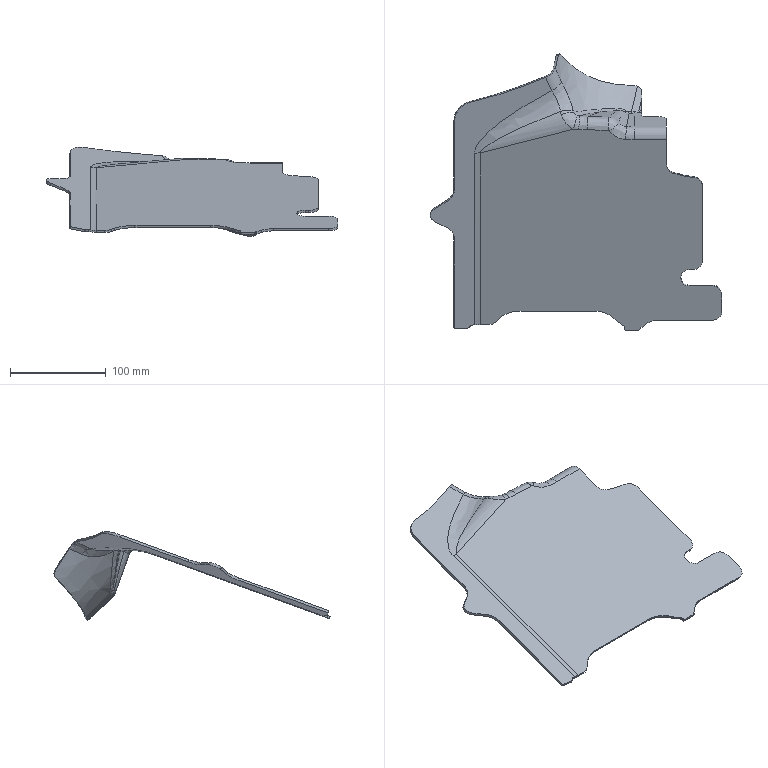Part | STEP file | lll_id182_x_t | 1 solid | 128 faces | box 305 x 288.456 x 93.297 mm | volume 170136 mm3 | spline 80 | plane 32 | cylinder 14 | torus 2 | commonest cylinder face diameters 1 x4 55 x2 16 x1 21 x1 50 x1 60 x1